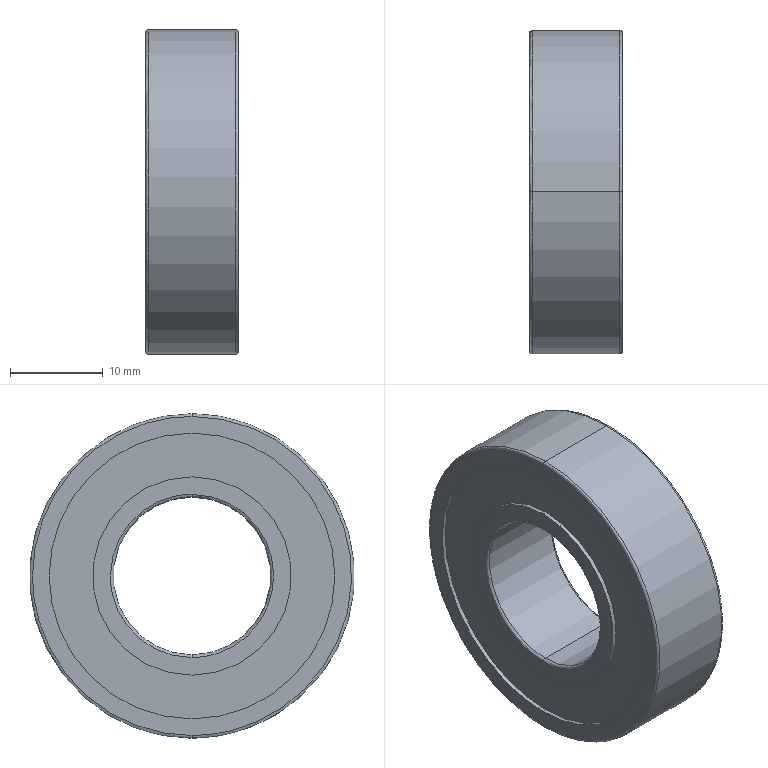Part | STEP file | B6003ZZ | 1 solid | 26 faces | box 10 x 35 x 35 mm | volume 7012 mm3 | cylinder 12 | spline 8 | plane 6 | commonest cylinder face diameters 21.4 x4 30.8 x4 17 x2 35 x2